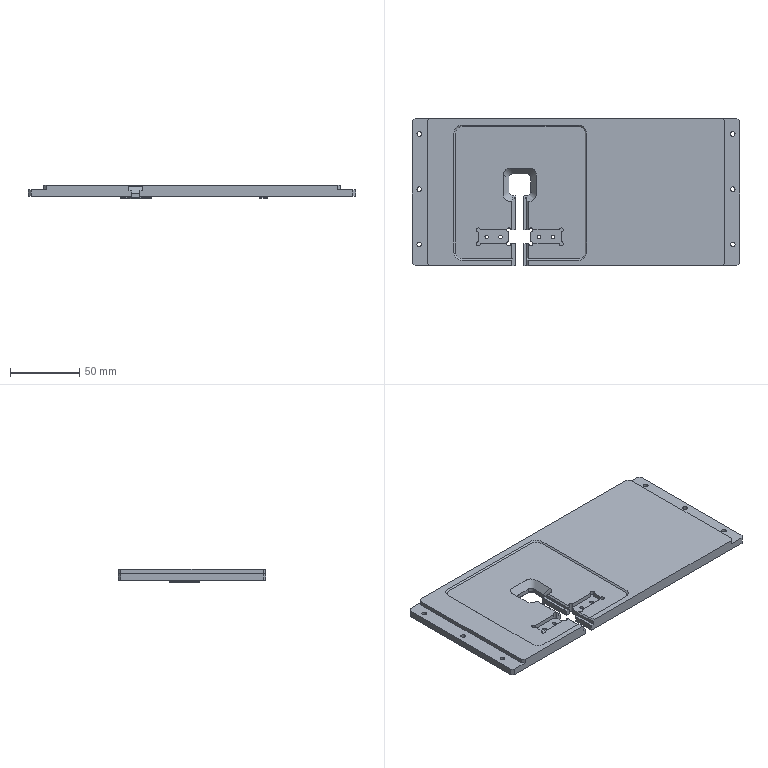Part | 1 solid | 294 faces | box 237 x 107 x 9.5 mm | volume 171061 mm3 | plane 151 | cylinder 70 | spline 51 | torus 12 | cone 8 | sphere 2 | commonest cylinder face diameters 1 x22 3 x12 3.3 x12 6 x12 2.5 x8 4 x4